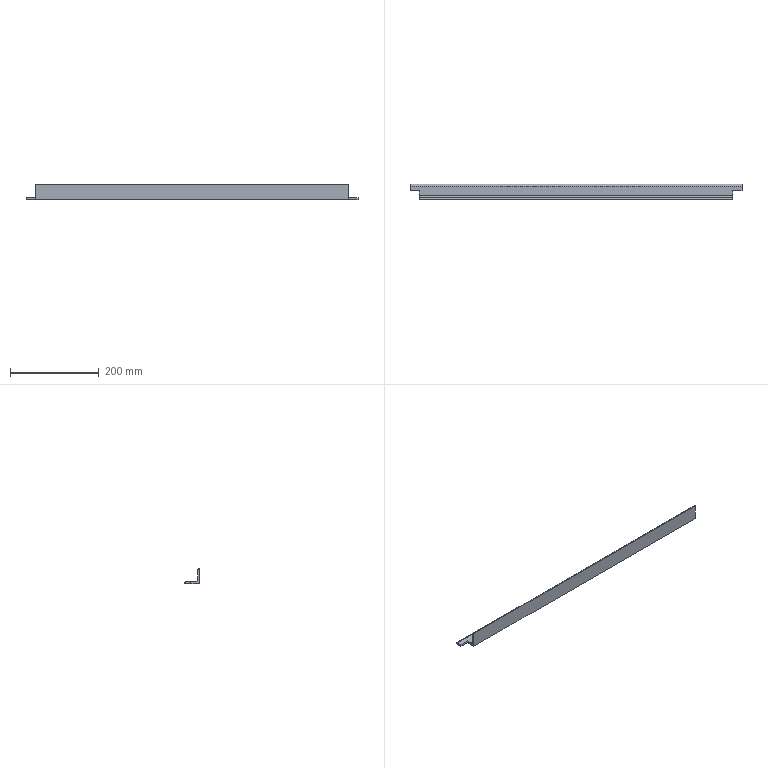Part | SolidWorks | features Cut 1, WeldMemberFeat 1, WeldmentFeature 1 | 1 solid | 13 faces | box 747 x 35 x 35 mm | volume 228267 mm3 | plane 10 | cylinder 3 | commonest cylinder face diameters 10 x3
STEP:
#1=CARTESIAN_POINT('',(747.,20.,0.));
#2=VERTEX_POINT('',#1);
#3=CARTESIAN_POINT('',(747.,35.,0.));
#4=VERTEX_POINT('',#3);
#5=CARTESIAN_POINT('',(747.,35.,0.));
#6=DIRECTION('',(0.,1.,0.));
#7=VECTOR('',#6,1000.);
#8=LINE('',#5,#7);
#9=EDGE_CURVE('',#2,#4,#8,.T.);
#10=ORIENTED_EDGE('',*,*,#9,.F.);
#11=CARTESIAN_POINT('',(726.,20.,0.));
#12=VERTEX_POINT('',#11);
#13=CARTESIAN_POINT('',(747.,20.,0.));
#14=DIRECTION('',(1.,0.,0.));
#15=VECTOR('',#14,1000.);
#16=LINE('',#13,#15);
#17=EDGE_CURVE('',#12,#2,#16,.T.);
#18=ORIENTED_EDGE('',*,*,#17,.F.);
#19=CARTESIAN_POINT('',(726.,0.,0.));
#20=VERTEX_POINT('',#19);
#21=CARTESIAN_POINT('',(726.,0.,0.));
#22=DIRECTION('',(0.,1.,0.));
#23=VECTOR('',#22,1000.);
#24=LINE('',#21,#23);
#25=EDGE_CURVE('',#20,#12,#24,.T.);
#26=ORIENTED_EDGE('',*,*,#25,.F.);
#27=CARTESIAN_POINT('',(21.,0.,0.));
#28=VERTEX_POINT('',#27);
#29=CARTESIAN_POINT('',(747.,0.,0.));
#30=DIRECTION('',(-1.,0.,0.));
#31=VECTOR('',#30,1000.);
#32=LINE('',#29,#31);
#33=EDGE_CURVE('',#20,#28,#32,.T.);
#34=ORIENTED_EDGE('',*,*,#33,.T.);
#35=CARTESIAN_POINT('',(21.,20.,0.));
#36=VERTEX_POINT('',#35);
#37=CARTESIAN_POINT('',(21.,0.,0.));
#38=DIRECTION('',(0.,-1.,0.));
#39=VECTOR('',#38,1000.);
#40=LINE('',#37,#39);
#41=EDGE_CURVE('',#36,#28,#40,.T.);
#42=ORIENTED_EDGE('',*,*,#41,.F.);
#43=CARTESIAN_POINT('',(0.,20.,0.));
#44=VERTEX_POINT('',#43);
#45=CARTESIAN_POINT('',(0.,20.,0.));
#46=DIRECTION('',(1.,0.,0.));
#47=VECTOR('',#46,1000.);
#48=LINE('',#45,#47);
#49=EDGE_CURVE('',#44,#36,#48,.T.);
#50=ORIENTED_EDGE('',*,*,#49,.F.);
#51=CARTESIAN_POINT('',(0.,35.,0.));
#52=VERTEX_POINT('',#51);
#53=CARTESIAN_POINT('',(0.,35.,0.));
#54=DIRECTION('',(0.,1.,0.));
#55=VECTOR('',#54,1000.);
#56=LINE('',#53,#55);
#57=EDGE_CURVE('',#44,#52,#56,.T.);
#58=ORIENTED_EDGE('',*,*,#57,.T.);
#59=CARTESIAN_POINT('',(747.,35.,0.));
#60=DIRECTION('',(-1.,0.,0.));
#61=VECTOR('',#60,1000.);
#62=LINE('',#59,#61);
#63=EDGE_CURVE('',#4,#52,#62,.T.);
#64=ORIENTED_EDGE('',*,*,#63,.F.);
#65=EDGE_LOOP('',(#10,#18,#26,#34,#42,#50,#58,#64));
#66=FACE_OUTER_BOUND('',#65,.T.);
#67=CARTESIAN_POINT('',(747.,35.,0.));
#68=DIRECTION('',(0.,0.,1.));
#69=DIRECTION('',(1.,0.,0.));
#70=AXIS2_PLACEMENT_3D('',#67,#68,#69);
#71=PLANE('',#70);
#72=ADVANCED_FACE('',(#66),#71,.F.);
#73=CARTESIAN_POINT('',(0.,30.,5.));
#74=VERTEX_POINT('',#73);
#75=CARTESIAN_POINT('',(0.,30.,0.));
#76=DIRECTION('',(1.,0.,0.));
#77=DIRECTION('',(0.,0.,-1.));
#78=AXIS2_PLACEMENT_3D('',#75,#76,#77);
#79=CIRCLE('',#78,5.);
#80=EDGE_CURVE('',#52,#74,#79,.T.);
#81=ORIENTED_EDGE('',*,*,#80,.T.);
#82=CARTESIAN_POINT('',(747.,30.,5.));
#83=VERTEX_POINT('',#82);
#84=CARTESIAN_POINT('',(747.,30.,5.));
#85=DIRECTION('',(-1.,0.,0.));
#86=VECTOR('',#85,1000.);
#87=LINE('',#84,#86);
#88=EDGE_CURVE('',#83,#74,#87,.T.);
#89=ORIENTED_EDGE('',*,*,#88,.F.);
#90=CARTESIAN_POINT('',(747.,30.,0.));
#91=DIRECTION('',(1.,0.,0.));
#92=DIRECTION('',(0.,0.,-1.));
#93=AXIS2_PLACEMENT_3D('',#90,#91,#92);
#94=CIRCLE('',#93,5.);
#95=EDGE_CURVE('',#4,#83,#94,.T.);
#96=ORIENTED_EDGE('',*,*,#95,.F.);
#97=ORIENTED_EDGE('',*,*,#63,.T.);
#98=EDGE_LOOP('',(#81,#89,#96,#97));
#99=FACE_OUTER_BOUND('',#98,.T.);
#100=CARTESIAN_POINT('',(747.,30.,0.));
#101=DIRECTION('',(-1.,0.,0.));
#102=DIRECTION('',(0.,0.,1.));
#103=AXIS2_PLACEMENT_3D('',#100,#101,#102);
#104=CYLINDRICAL_SURFACE('',#103,5.);
#105=ADVANCED_FACE('',(#99),#104,.T.);
#106=CARTESIAN_POINT('',(726.,10.,5.));
#107=VERTEX_POINT('',#106);
#108=CARTESIAN_POINT('',(726.,20.,5.));
#109=VERTEX_POINT('',#108);
#110=CARTESIAN_POINT('',(726.,10.,5.));
#111=DIRECTION('',(0.,1.,0.));
#112=VECTOR('',#111,1000.);
#113=LINE('',#110,#112);
#114=EDGE_CURVE('',#107,#109,#113,.T.);
#115=ORIENTED_EDGE('',*,*,#114,.T.);
#116=CARTESIAN_POINT('',(747.,20.,5.));
#117=VERTEX_POINT('',#116);
#118=CARTESIAN_POINT('',(747.,20.,5.));
#119=DIRECTION('',(1.,0.,0.));
#120=VECTOR('',#119,1000.);
#121=LINE('',#118,#120);
#122=EDGE_CURVE('',#109,#117,#121,.T.);
#123=ORIENTED_EDGE('',*,*,#122,.T.);
#124=CARTESIAN_POINT('',(747.,10.,5.));
#125=DIRECTION('',(0.,-1.,0.));
#126=VECTOR('',#125,1000.);
#127=LINE('',#124,#126);
#128=EDGE_CURVE('',#83,#117,#127,.T.);
#129=ORIENTED_EDGE('',*,*,#128,.F.);
#130=ORIENTED_EDGE('',*,*,#88,.T.);
#131=CARTESIAN_POINT('',(0.,20.,5.));
#132=VERTEX_POINT('',#131);
#133=CARTESIAN_POINT('',(0.,10.,5.));
#134=DIRECTION('',(0.,-1.,0.));
#135=VECTOR('',#134,1000.);
#136=LINE('',#133,#135);
#137=EDGE_CURVE('',#74,#132,#136,.T.);
#138=ORIENTED_EDGE('',*,*,#137,.T.);
#139=CARTESIAN_POINT('',(21.,20.,5.));
#140=VERTEX_POINT('',#139);
#141=CARTESIAN_POINT('',(747.,20.,5.));
#142=DIRECTION('',(1.,0.,0.));
#143=VECTOR('',#142,1000.);
#144=LINE('',#141,#143);
#145=EDGE_CURVE('',#132,#140,#144,.T.);
#146=ORIENTED_EDGE('',*,*,#145,.T.);
#147=CARTESIAN_POINT('',(21.,10.,5.));
#148=VERTEX_POINT('',#147);
#149=CARTESIAN_POINT('',(21.,10.,5.));
#150=DIRECTION('',(0.,-1.,0.));
#151=VECTOR('',#150,1000.);
#152=LINE('',#149,#151);
#153=EDGE_CURVE('',#140,#148,#152,.T.);
#154=ORIENTED_EDGE('',*,*,#153,.T.);
#155=CARTESIAN_POINT('',(747.,10.,5.));
#156=DIRECTION('',(-1.,0.,0.));
#157=VECTOR('',#156,1000.);
#158=LINE('',#155,#157);
#159=EDGE_CURVE('',#107,#148,#158,.T.);
#160=ORIENTED_EDGE('',*,*,#159,.F.);
#161=EDGE_LOOP('',(#115,#123,#129,#130,#138,#146,#154,#160));
#162=FACE_OUTER_BOUND('',#161,.T.);
#163=CARTESIAN_POINT('',(747.,10.,5.));
#164=DIRECTION('',(0.,0.,-1.));
#165=DIRECTION('',(0.,1.,0.));
#166=AXIS2_PLACEMENT_3D('',#163,#164,#165);
#167=PLANE('',#166);
#168=ADVANCED_FACE('',(#162),#167,.F.);
#169=CARTESIAN_POINT('',(726.,5.,10.));
#170=VERTEX_POINT('',#169);
#171=CARTESIAN_POINT('',(21.,5.,10.));
#172=VERTEX_POINT('',#171);
#173=CARTESIAN_POINT('',(747.,5.,10.));
#174=DIRECTION('',(-1.,0.,0.));
#175=VECTOR('',#174,1000.);
#176=LINE('',#173,#175);
#177=EDGE_CURVE('',#170,#172,#176,.T.);
#178=ORIENTED_EDGE('',*,*,#177,.F.);
#179=CARTESIAN_POINT('',(726.,10.,10.));
#180=DIRECTION('',(1.,0.,0.));
#181=DIRECTION('',(0.,0.,1.));
#182=AXIS2_PLACEMENT_3D('',#179,#180,#181);
#183=CIRCLE('',#182,5.);
#184=EDGE_CURVE('',#170,#107,#183,.T.);
#185=ORIENTED_EDGE('',*,*,#184,.T.);
#186=ORIENTED_EDGE('',*,*,#159,.T.);
#187=CARTESIAN_POINT('',(21.,10.,10.));
#188=DIRECTION('',(-1.,0.,0.));
#189=DIRECTION('',(0.,0.,-1.));
#190=AXIS2_PLACEMENT_3D('',#187,#188,#189);
#191=CIRCLE('',#190,5.);
#192=EDGE_CURVE('',#148,#172,#191,.T.);
#193=ORIENTED_EDGE('',*,*,#192,.T.);
#194=EDGE_LOOP('',(#178,#185,#186,#193));
#195=FACE_OUTER_BOUND('',#194,.T.);
#196=CARTESIAN_POINT('',(747.,10.,10.));
#197=DIRECTION('',(-1.,0.,0.));
#198=DIRECTION('',(0.,0.,1.));
#199=AXIS2_PLACEMENT_3D('',#196,#197,#198);
#200=CYLINDRICAL_SURFACE('',#199,5.);
#201=ADVANCED_FACE('',(#195),#200,.F.);
#202=CARTESIAN_POINT('',(726.,5.,30.));
#203=VERTEX_POINT('',#202);
#204=CARTESIAN_POINT('',(21.,5.,30.));
#205=VERTEX_POINT('',#204);
#206=CARTESIAN_POINT('',(747.,5.,30.));
#207=DIRECTION('',(-1.,0.,0.));
#208=VECTOR('',#207,1000.);
#209=LINE('',#206,#208);
#210=EDGE_CURVE('',#203,#205,#209,.T.);
#211=ORIENTED_EDGE('',*,*,#210,.F.);
#212=CARTESIAN_POINT('',(726.,5.,30.));
#213=DIRECTION('',(0.,0.,-1.));
#214=VECTOR('',#213,1000.);
#215=LINE('',#212,#214);
#216=EDGE_CURVE('',#203,#170,#215,.T.);
#217=ORIENTED_EDGE('',*,*,#216,.T.);
#218=ORIENTED_EDGE('',*,*,#177,.T.);
#219=CARTESIAN_POINT('',(21.,5.,30.));
#220=DIRECTION('',(0.,0.,1.));
#221=VECTOR('',#220,1000.);
#222=LINE('',#219,#221);
#223=EDGE_CURVE('',#172,#205,#222,.T.);
#224=ORIENTED_EDGE('',*,*,#223,.T.);
#225=EDGE_LOOP('',(#211,#217,#218,#224));
#226=FACE_OUTER_BOUND('',#225,.T.);
#227=CARTESIAN_POINT('',(747.,5.,30.));
#228=DIRECTION('',(0.,-1.,0.));
#229=DIRECTION('',(0.,0.,-1.));
#230=AXIS2_PLACEMENT_3D('',#227,#228,#229);
#231=PLANE('',#230);
#232=ADVANCED_FACE('',(#226),#231,.F.);
#233=CARTESIAN_POINT('',(726.,0.,35.));
#234=VERTEX_POINT('',#233);
#235=CARTESIAN_POINT('',(21.,0.,35.));
#236=VERTEX_POINT('',#235);
#237=CARTESIAN_POINT('',(747.,0.,35.));
#238=DIRECTION('',(-1.,0.,0.));
#239=VECTOR('',#238,1000.);
#240=LINE('',#237,#239);
#241=EDGE_CURVE('',#234,#236,#240,.T.);
#242=ORIENTED_EDGE('',*,*,#241,.F.);
#243=CARTESIAN_POINT('',(726.,0.,30.));
#244=DIRECTION('',(-1.,0.,0.));
#245=DIRECTION('',(0.,0.,1.));
#246=AXIS2_PLACEMENT_3D('',#243,#244,#245);
#247=CIRCLE('',#246,5.);
#248=EDGE_CURVE('',#234,#203,#247,.T.);
#249=ORIENTED_EDGE('',*,*,#248,.T.);
#250=ORIENTED_EDGE('',*,*,#210,.T.);
#251=CARTESIAN_POINT('',(21.,0.,30.));
#252=DIRECTION('',(1.,0.,0.));
#253=DIRECTION('',(0.,0.,-1.));
#254=AXIS2_PLACEMENT_3D('',#251,#252,#253);
#255=CIRCLE('',#254,5.);
#256=EDGE_CURVE('',#205,#236,#255,.T.);
#257=ORIENTED_EDGE('',*,*,#256,.T.);
#258=EDGE_LOOP('',(#242,#249,#250,#257));
#259=FACE_OUTER_BOUND('',#258,.T.);
#260=CARTESIAN_POINT('',(747.,0.,30.));
#261=DIRECTION('',(-1.,0.,0.));
#262=DIRECTION('',(0.,0.,1.));
#263=AXIS2_PLACEMENT_3D('',#260,#261,#262);
#264=CYLINDRICAL_SURFACE('',#263,5.);
#265=ADVANCED_FACE('',(#259),#264,.T.);
#266=ORIENTED_EDGE('',*,*,#33,.F.);
#267=CARTESIAN_POINT('',(726.,0.,35.));
#268=DIRECTION('',(0.,0.,-1.));
#269=VECTOR('',#268,1000.);
#270=LINE('',#267,#269);
#271=EDGE_CURVE('',#234,#20,#270,.T.);
#272=ORIENTED_EDGE('',*,*,#271,.F.);
#273=ORIENTED_EDGE('',*,*,#241,.T.);
#274=CARTESIAN_POINT('',(21.,0.,35.));
#275=DIRECTION('',(0.,0.,-1.));
#276=VECTOR('',#275,1000.);
#277=LINE('',#274,#276);
#278=EDGE_CURVE('',#236,#28,#277,.T.);
#279=ORIENTED_EDGE('',*,*,#278,.T.);
#280=EDGE_LOOP('',(#266,#272,#273,#279));
#281=FACE_OUTER_BOUND('',#280,.T.);
#282=CARTESIAN_POINT('',(747.,0.,0.));
#283=DIRECTION('',(0.,1.,0.));
#284=DIRECTION('',(0.,0.,1.));
#285=AXIS2_PLACEMENT_3D('',#282,#283,#284);
#286=PLANE('',#285);
#287=ADVANCED_FACE('',(#281),#286,.F.);
#288=ORIENTED_EDGE('',*,*,#128,.T.);
#289=CARTESIAN_POINT('',(747.,20.,30.));
#290=DIRECTION('',(0.,0.,-1.));
#291=VECTOR('',#290,1000.);
#292=LINE('',#289,#291);
#293=EDGE_CURVE('',#117,#2,#292,.T.);
#294=ORIENTED_EDGE('',*,*,#293,.T.);
#295=ORIENTED_EDGE('',*,*,#9,.T.);
#296=ORIENTED_EDGE('',*,*,#95,.T.);
#297=EDGE_LOOP('',(#288,#294,#295,#296));
#298=FACE_OUTER_BOUND('',#297,.T.);
#299=CARTESIAN_POINT('',(747.,0.,30.));
#300=DIRECTION('',(-1.,0.,0.));
#301=DIRECTION('',(0.,0.,1.));
#302=AXIS2_PLACEMENT_3D('',#299,#300,#301);
#303=PLANE('',#302);
#304=ADVANCED_FACE('',(#298),#303,.F.);
#305=CARTESIAN_POINT('',(0.,20.,30.));
#306=DIRECTION('',(0.,0.,-1.));
#307=VECTOR('',#306,1000.);
#308=LINE('',#305,#307);
#309=EDGE_CURVE('',#132,#44,#308,.T.);
#310=ORIENTED_EDGE('',*,*,#309,.F.);
#311=ORIENTED_EDGE('',*,*,#137,.F.);
#312=ORIENTED_EDGE('',*,*,#80,.F.);
#313=ORIENTED_EDGE('',*,*,#57,.F.);
#314=EDGE_LOOP('',(#310,#311,#312,#313));
#315=FACE_OUTER_BOUND('',#314,.T.);
#316=CARTESIAN_POINT('',(0.,0.,30.));
#317=DIRECTION('',(-1.,0.,0.));
#318=DIRECTION('',(0.,0.,1.));
#319=AXIS2_PLACEMENT_3D('',#316,#317,#318);
#320=PLANE('',#319);
#321=ADVANCED_FACE('',(#315),#320,.T.);
#322=CARTESIAN_POINT('',(21.,20.,35.));
#323=DIRECTION('',(0.,0.,-1.));
#324=VECTOR('',#323,1000.);
#325=LINE('',#322,#324);
#326=EDGE_CURVE('',#140,#36,#325,.T.);
#327=ORIENTED_EDGE('',*,*,#326,.T.);
#328=ORIENTED_EDGE('',*,*,#41,.T.);
#329=ORIENTED_EDGE('',*,*,#278,.F.);
#330=ORIENTED_EDGE('',*,*,#256,.F.);
#331=ORIENTED_EDGE('',*,*,#223,.F.);
#332=ORIENTED_EDGE('',*,*,#192,.F.);
#333=ORIENTED_EDGE('',*,*,#153,.F.);
#334=EDGE_LOOP('',(#327,#328,#329,#330,#331,#332,#333));
#335=FACE_OUTER_BOUND('',#334,.T.);
#336=CARTESIAN_POINT('',(21.,0.,35.));
#337=DIRECTION('',(1.,0.,0.));
#338=DIRECTION('',(0.,0.,-1.));
#339=AXIS2_PLACEMENT_3D('',#336,#337,#338);
#340=PLANE('',#339);
#341=ADVANCED_FACE('',(#335),#340,.F.);
#342=ORIENTED_EDGE('',*,*,#309,.T.);
#343=ORIENTED_EDGE('',*,*,#49,.T.);
#344=ORIENTED_EDGE('',*,*,#326,.F.);
#345=ORIENTED_EDGE('',*,*,#145,.F.);
#346=EDGE_LOOP('',(#342,#343,#344,#345));
#347=FACE_OUTER_BOUND('',#346,.T.);
#348=CARTESIAN_POINT('',(0.,20.,35.));
#349=DIRECTION('',(0.,1.,0.));
#350=DIRECTION('',(-1.,0.,0.));
#351=AXIS2_PLACEMENT_3D('',#348,#349,#350);
#352=PLANE('',#351);
#353=ADVANCED_FACE('',(#347),#352,.F.);
#354=ORIENTED_EDGE('',*,*,#184,.F.);
#355=ORIENTED_EDGE('',*,*,#216,.F.);
#356=ORIENTED_EDGE('',*,*,#248,.F.);
#357=ORIENTED_EDGE('',*,*,#271,.T.);
#358=ORIENTED_EDGE('',*,*,#25,.T.);
#359=CARTESIAN_POINT('',(726.,20.,35.));
#360=DIRECTION('',(0.,0.,-1.));
#361=VECTOR('',#360,1000.);
#362=LINE('',#359,#361);
#363=EDGE_CURVE('',#109,#12,#362,.T.);
#364=ORIENTED_EDGE('',*,*,#363,.F.);
#365=ORIENTED_EDGE('',*,*,#114,.F.);
#366=EDGE_LOOP('',(#354,#355,#356,#357,#358,#364,#365));
#367=FACE_OUTER_BOUND('',#366,.T.);
#368=CARTESIAN_POINT('',(726.,0.,35.));
#369=DIRECTION('',(-1.,0.,0.));
#370=DIRECTION('',(0.,0.,1.));
#371=AXIS2_PLACEMENT_3D('',#368,#369,#370);
#372=PLANE('',#371);
#373=ADVANCED_FACE('',(#367),#372,.F.);
#374=ORIENTED_EDGE('',*,*,#363,.T.);
#375=ORIENTED_EDGE('',*,*,#17,.T.);
#376=ORIENTED_EDGE('',*,*,#293,.F.);
#377=ORIENTED_EDGE('',*,*,#122,.F.);
#378=EDGE_LOOP('',(#374,#375,#376,#377));
#379=FACE_OUTER_BOUND('',#378,.T.);
#380=CARTESIAN_POINT('',(747.,20.,35.));
#381=DIRECTION('',(0.,1.,0.));
#382=DIRECTION('',(0.,0.,1.));
#383=AXIS2_PLACEMENT_3D('',#380,#381,#382);
#384=PLANE('',#383);
#385=ADVANCED_FACE('',(#379),#384,.F.);
#386=CLOSED_SHELL('',(#72,#105,#168,#201,#232,#265,#287,#304,#321,#341,#353,#373,#385));
#387=MANIFOLD_SOLID_BREP('',#386);
#388=CARTESIAN_POINT('',(0.,0.,0.));
#389=DIRECTION('',(0.,0.,1.));
#390=DIRECTION('',(1.,0.,0.));
#391=AXIS2_PLACEMENT_3D('',#388,#389,#390);
#392=(LENGTH_UNIT()NAMED_UNIT(*)SI_UNIT(.MILLI.,.METRE.));
#393=UNCERTAINTY_MEASURE_WITH_UNIT(LENGTH_MEASURE(0.00001),#392,'','');
#394=(NAMED_UNIT(*)PLANE_ANGLE_UNIT()SI_UNIT($,.RADIAN.));
#395=(NAMED_UNIT(*)SI_UNIT($,.STERADIAN.)SOLID_ANGLE_UNIT());
#396=(GEOMETRIC_REPRESENTATION_CONTEXT(3)GLOBAL_UNCERTAINTY_ASSIGNED_CONTEXT((#393))GLOBAL_UNIT_ASSIGNED_CONTEXT((#392,#394,#395))REPRESENTATION_CONTEXT('',''));
#397=ADVANCED_BREP_SHAPE_REPRESENTATION('',(#387,#391),#396);